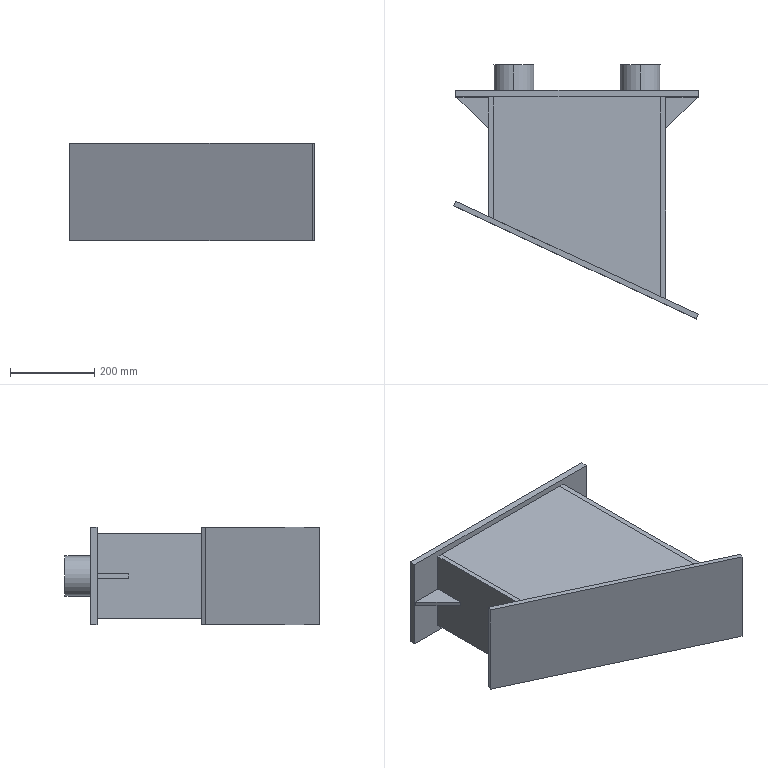Part | STEP file | Spring lower seat 1_Default<As machined> | 10 solids | 58 faces | box 580.577 x 601.953 x 230 mm | volume 9576180 mm3 | plane 50 | cylinder 8 | commonest cylinder face diameters 83 x4 95 x4